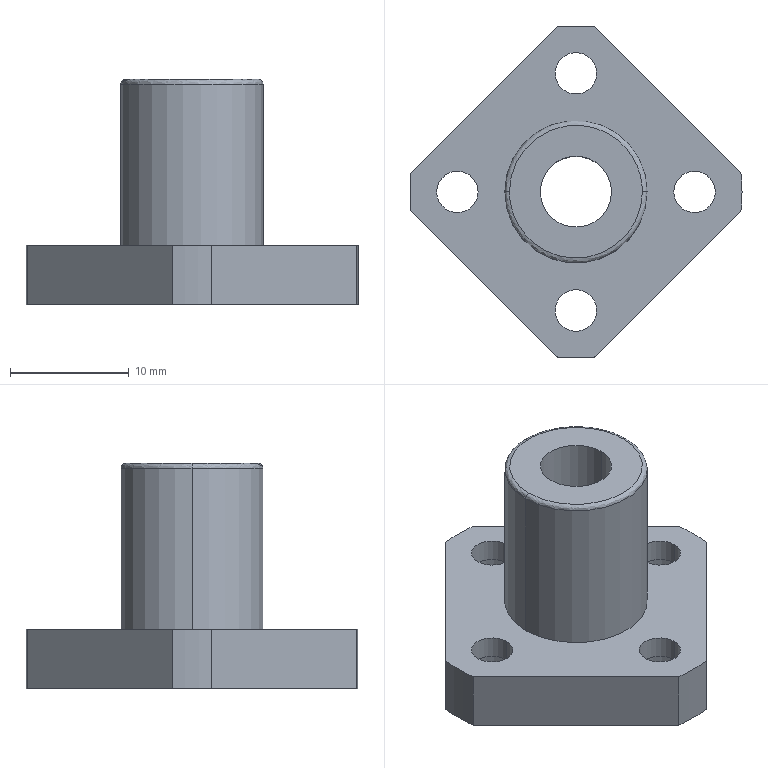Part | SolidWorks | features BaseBody 1 | 1 solid | 38 faces | box 28 x 28 x 19 mm | volume 2991 mm3 | cylinder 25 | plane 11 | spline 2 | commonest cylinder face diameters 6 x10 3.5 x8 28 x5 12 x2
STEP:
#1=CARTESIAN_POINT('',(6.,0.,18.6));
#2=VERTEX_POINT('',#1);
#3=CARTESIAN_POINT('',(-6.,0.,18.6));
#4=VERTEX_POINT('',#3);
#5=CARTESIAN_POINT('',(0.,0.,18.6));
#6=DIRECTION('',(0.,0.,-1.));
#7=DIRECTION('',(1.,0.,0.));
#8=AXIS2_PLACEMENT_3D('',#5,#6,#7);
#9=CIRCLE('',#8,6.);
#10=EDGE_CURVE('',#2,#4,#9,.T.);
#11=ORIENTED_EDGE('',*,*,#10,.F.);
#12=CARTESIAN_POINT('',(5.6,0.,19.));
#13=VERTEX_POINT('',#12);
#14=CARTESIAN_POINT('',(5.6,0.,18.6));
#15=DIRECTION('',(0.,-1.,0.));
#16=DIRECTION('',(1.,0.,0.));
#17=AXIS2_PLACEMENT_3D('',#14,#15,#16);
#18=CIRCLE('',#17,0.4);
#19=EDGE_CURVE('',#2,#13,#18,.T.);
#20=ORIENTED_EDGE('',*,*,#19,.T.);
#21=CARTESIAN_POINT('',(-5.6,0.,19.));
#22=VERTEX_POINT('',#21);
#23=CARTESIAN_POINT('',(5.6,0.,19.));
#24=CARTESIAN_POINT('',(5.6,-11.2,19.));
#25=CARTESIAN_POINT('',(-5.6,-11.2,19.));
#26=CARTESIAN_POINT('',(-5.6,0.,19.));
#27=(BOUNDED_CURVE()B_SPLINE_CURVE(3,(#23,#24,#25,#26),.UNSPECIFIED.,.F.,.T.)B_SPLINE_CURVE_WITH_KNOTS((4,4),(0.5,1.),.UNSPECIFIED.)CURVE()GEOMETRIC_REPRESENTATION_ITEM()RATIONAL_B_SPLINE_CURVE((1.,0.3333,0.3333,1.))REPRESENTATION_ITEM(''));
#28=EDGE_CURVE('',#13,#22,#27,.T.);
#29=ORIENTED_EDGE('',*,*,#28,.T.);
#30=CARTESIAN_POINT('',(-5.6,0.,18.6));
#31=DIRECTION('',(0.,1.,0.));
#32=DIRECTION('',(-1.,0.,0.));
#33=AXIS2_PLACEMENT_3D('',#30,#31,#32);
#34=CIRCLE('',#33,0.4);
#35=EDGE_CURVE('',#4,#22,#34,.T.);
#36=ORIENTED_EDGE('',*,*,#35,.F.);
#37=EDGE_LOOP('',(#11,#20,#29,#36));
#38=FACE_OUTER_BOUND('',#37,.T.);
#39=CARTESIAN_POINT('',(6.,0.,18.6));
#40=CARTESIAN_POINT('',(6.,-12.,18.6));
#41=CARTESIAN_POINT('',(-6.,-12.,18.6));
#42=CARTESIAN_POINT('',(-6.,0.,18.6));
#43=CARTESIAN_POINT('',(6.,0.,18.834));
#44=CARTESIAN_POINT('',(6.,-12.,18.834));
#45=CARTESIAN_POINT('',(-6.,-12.,18.834));
#46=CARTESIAN_POINT('',(-6.,0.,18.834));
#47=CARTESIAN_POINT('',(5.834,0.,19.));
#48=CARTESIAN_POINT('',(5.834,-11.669,19.));
#49=CARTESIAN_POINT('',(-5.834,-11.669,19.));
#50=CARTESIAN_POINT('',(-5.834,0.,19.));
#51=CARTESIAN_POINT('',(5.6,0.,19.));
#52=CARTESIAN_POINT('',(5.6,-11.2,19.));
#53=CARTESIAN_POINT('',(-5.6,-11.2,19.));
#54=CARTESIAN_POINT('',(-5.6,0.,19.));
#55=(BOUNDED_SURFACE()B_SPLINE_SURFACE(3,3,((#39,#40,#41,#42),(#43,#44,#45,#46),(#47,#48,#49,#50),(#51,#52,#53,#54)),.UNSPECIFIED.,.F.,.F.,.F.)B_SPLINE_SURFACE_WITH_KNOTS((4,4),(4,4),(0.,1.),(0.,1.),.UNSPECIFIED.)GEOMETRIC_REPRESENTATION_ITEM()RATIONAL_B_SPLINE_SURFACE(((1.,0.3333,0.3333,1.),(0.8047,0.2682,0.2682,0.8047),(0.8047,0.2682,0.2682,0.8047),(1.,0.3333,0.3333,1.)))REPRESENTATION_ITEM('')SURFACE());
#56=ADVANCED_FACE('',(#38),#55,.T.);
#57=CARTESIAN_POINT('',(6.,0.,5.));
#58=VERTEX_POINT('',#57);
#59=CARTESIAN_POINT('',(-6.,0.,5.));
#60=VERTEX_POINT('',#59);
#61=CARTESIAN_POINT('',(0.,0.,5.));
#62=DIRECTION('',(0.,0.,1.));
#63=DIRECTION('',(1.,0.,0.));
#64=AXIS2_PLACEMENT_3D('',#61,#62,#63);
#65=CIRCLE('',#64,6.);
#66=EDGE_CURVE('',#58,#60,#65,.T.);
#67=ORIENTED_EDGE('',*,*,#66,.T.);
#68=CARTESIAN_POINT('',(-6.,0.,0.));
#69=DIRECTION('',(0.,0.,1.));
#70=VECTOR('',#69,1000.);
#71=LINE('',#68,#70);
#72=EDGE_CURVE('',#60,#4,#71,.T.);
#73=ORIENTED_EDGE('',*,*,#72,.T.);
#74=CARTESIAN_POINT('',(0.,0.,18.6));
#75=DIRECTION('',(0.,0.,-1.));
#76=DIRECTION('',(1.,0.,0.));
#77=AXIS2_PLACEMENT_3D('',#74,#75,#76);
#78=CIRCLE('',#77,6.);
#79=EDGE_CURVE('',#4,#2,#78,.T.);
#80=ORIENTED_EDGE('',*,*,#79,.T.);
#81=CARTESIAN_POINT('',(6.,0.,0.));
#82=DIRECTION('',(0.,0.,1.));
#83=VECTOR('',#82,1000.);
#84=LINE('',#81,#83);
#85=EDGE_CURVE('',#58,#2,#84,.T.);
#86=ORIENTED_EDGE('',*,*,#85,.F.);
#87=EDGE_LOOP('',(#67,#73,#80,#86));
#88=FACE_OUTER_BOUND('',#87,.T.);
#89=CARTESIAN_POINT('',(0.,0.,0.));
#90=DIRECTION('',(0.,0.,1.));
#91=DIRECTION('',(1.,0.,0.));
#92=AXIS2_PLACEMENT_3D('',#89,#90,#91);
#93=CYLINDRICAL_SURFACE('',#92,6.);
#94=ADVANCED_FACE('',(#88),#93,.T.);
#95=CARTESIAN_POINT('',(-1.75,10.,3.1));
#96=VERTEX_POINT('',#95);
#97=CARTESIAN_POINT('',(1.75,10.,3.1));
#98=VERTEX_POINT('',#97);
#99=CARTESIAN_POINT('',(0.,10.,3.1));
#100=DIRECTION('',(0.,0.,1.));
#101=DIRECTION('',(1.,0.,0.));
#102=AXIS2_PLACEMENT_3D('',#99,#100,#101);
#103=CIRCLE('',#102,1.75);
#104=EDGE_CURVE('',#96,#98,#103,.T.);
#105=ORIENTED_EDGE('',*,*,#104,.F.);
#106=CARTESIAN_POINT('',(-1.75,10.,5.));
#107=VERTEX_POINT('',#106);
#108=CARTESIAN_POINT('',(-1.75,10.,0.));
#109=DIRECTION('',(0.,0.,1.));
#110=VECTOR('',#109,1000.);
#111=LINE('',#108,#110);
#112=EDGE_CURVE('',#96,#107,#111,.T.);
#113=ORIENTED_EDGE('',*,*,#112,.T.);
#114=CARTESIAN_POINT('',(1.75,10.,5.));
#115=VERTEX_POINT('',#114);
#116=CARTESIAN_POINT('',(0.,10.,5.));
#117=DIRECTION('',(0.,0.,-1.));
#118=DIRECTION('',(1.,0.,0.));
#119=AXIS2_PLACEMENT_3D('',#116,#117,#118);
#120=CIRCLE('',#119,1.75);
#121=EDGE_CURVE('',#115,#107,#120,.T.);
#122=ORIENTED_EDGE('',*,*,#121,.F.);
#123=CARTESIAN_POINT('',(1.75,10.,0.));
#124=DIRECTION('',(0.,0.,1.));
#125=VECTOR('',#124,1000.);
#126=LINE('',#123,#125);
#127=EDGE_CURVE('',#98,#115,#126,.T.);
#128=ORIENTED_EDGE('',*,*,#127,.F.);
#129=EDGE_LOOP('',(#105,#113,#122,#128));
#130=FACE_OUTER_BOUND('',#129,.T.);
#131=CARTESIAN_POINT('',(0.,10.,0.));
#132=DIRECTION('',(0.,0.,1.));
#133=DIRECTION('',(1.,0.,0.));
#134=AXIS2_PLACEMENT_3D('',#131,#132,#133);
#135=CYLINDRICAL_SURFACE('',#134,1.75);
#136=ADVANCED_FACE('',(#130),#135,.F.);
#137=CARTESIAN_POINT('',(11.75,0.,5.));
#138=VERTEX_POINT('',#137);
#139=CARTESIAN_POINT('',(8.25,0.,5.));
#140=VERTEX_POINT('',#139);
#141=CARTESIAN_POINT('',(10.,0.,5.));
#142=DIRECTION('',(0.,0.,-1.));
#143=DIRECTION('',(-1.,0.,0.));
#144=AXIS2_PLACEMENT_3D('',#141,#142,#143);
#145=CIRCLE('',#144,1.75);
#146=EDGE_CURVE('',#138,#140,#145,.T.);
#147=ORIENTED_EDGE('',*,*,#146,.F.);
#148=CARTESIAN_POINT('',(11.75,0.,3.1));
#149=VERTEX_POINT('',#148);
#150=CARTESIAN_POINT('',(11.75,0.,5.));
#151=DIRECTION('',(0.,0.,-1.));
#152=VECTOR('',#151,1000.);
#153=LINE('',#150,#152);
#154=EDGE_CURVE('',#138,#149,#153,.T.);
#155=ORIENTED_EDGE('',*,*,#154,.T.);
#156=CARTESIAN_POINT('',(8.25,0.,3.1));
#157=VERTEX_POINT('',#156);
#158=CARTESIAN_POINT('',(10.,0.,3.1));
#159=DIRECTION('',(0.,0.,1.));
#160=DIRECTION('',(-1.,0.,0.));
#161=AXIS2_PLACEMENT_3D('',#158,#159,#160);
#162=CIRCLE('',#161,1.75);
#163=EDGE_CURVE('',#157,#149,#162,.T.);
#164=ORIENTED_EDGE('',*,*,#163,.F.);
#165=CARTESIAN_POINT('',(8.25,0.,5.));
#166=DIRECTION('',(0.,0.,-1.));
#167=VECTOR('',#166,1000.);
#168=LINE('',#165,#167);
#169=EDGE_CURVE('',#140,#157,#168,.T.);
#170=ORIENTED_EDGE('',*,*,#169,.F.);
#171=EDGE_LOOP('',(#147,#155,#164,#170));
#172=FACE_OUTER_BOUND('',#171,.T.);
#173=CARTESIAN_POINT('',(10.,0.,5.));
#174=DIRECTION('',(0.,0.,-1.));
#175=DIRECTION('',(-1.,0.,0.));
#176=AXIS2_PLACEMENT_3D('',#173,#174,#175);
#177=CYLINDRICAL_SURFACE('',#176,1.75);
#178=ADVANCED_FACE('',(#172),#177,.F.);
#179=CARTESIAN_POINT('',(13.902,-1.654,0.));
#180=VERTEX_POINT('',#179);
#181=CARTESIAN_POINT('',(14.,0.,0.));
#182=VERTEX_POINT('',#181);
#183=CARTESIAN_POINT('',(0.,0.,0.));
#184=DIRECTION('',(0.,0.,1.));
#185=DIRECTION('',(1.,0.,0.));
#186=AXIS2_PLACEMENT_3D('',#183,#184,#185);
#187=CIRCLE('',#186,14.);
#188=EDGE_CURVE('',#180,#182,#187,.T.);
#189=ORIENTED_EDGE('',*,*,#188,.T.);
#190=CARTESIAN_POINT('',(14.,0.,5.));
#191=VERTEX_POINT('',#190);
#192=CARTESIAN_POINT('',(14.,0.,5.));
#193=DIRECTION('',(0.,0.,1.));
#194=VECTOR('',#193,1000.);
#195=LINE('',#192,#194);
#196=EDGE_CURVE('',#182,#191,#195,.T.);
#197=ORIENTED_EDGE('',*,*,#196,.T.);
#198=CARTESIAN_POINT('',(13.902,-1.654,5.));
#199=VERTEX_POINT('',#198);
#200=CARTESIAN_POINT('',(0.,0.,5.));
#201=DIRECTION('',(0.,0.,1.));
#202=DIRECTION('',(1.,0.,0.));
#203=AXIS2_PLACEMENT_3D('',#200,#201,#202);
#204=CIRCLE('',#203,14.);
#205=EDGE_CURVE('',#199,#191,#204,.T.);
#206=ORIENTED_EDGE('',*,*,#205,.F.);
#207=CARTESIAN_POINT('',(13.902,-1.654,5.));
#208=DIRECTION('',(0.,0.,-1.));
#209=VECTOR('',#208,1000.);
#210=LINE('',#207,#209);
#211=EDGE_CURVE('',#199,#180,#210,.T.);
#212=ORIENTED_EDGE('',*,*,#211,.T.);
#213=EDGE_LOOP('',(#189,#197,#206,#212));
#214=FACE_OUTER_BOUND('',#213,.T.);
#215=CARTESIAN_POINT('',(0.,0.,5.));
#216=DIRECTION('',(0.,0.,1.));
#217=DIRECTION('',(1.,0.,0.));
#218=AXIS2_PLACEMENT_3D('',#215,#216,#217);
#219=CYLINDRICAL_SURFACE('',#218,14.);
#220=ADVANCED_FACE('',(#214),#219,.T.);
#221=CARTESIAN_POINT('',(-11.75,0.,3.1));
#222=VERTEX_POINT('',#221);
#223=CARTESIAN_POINT('',(-8.25,0.,3.1));
#224=VERTEX_POINT('',#223);
#225=CARTESIAN_POINT('',(-10.,0.,3.1));
#226=DIRECTION('',(0.,0.,1.));
#227=DIRECTION('',(1.,0.,0.));
#228=AXIS2_PLACEMENT_3D('',#225,#226,#227);
#229=CIRCLE('',#228,1.75);
#230=EDGE_CURVE('',#222,#224,#229,.T.);
#231=ORIENTED_EDGE('',*,*,#230,.F.);
#232=CARTESIAN_POINT('',(-11.75,0.,5.));
#233=VERTEX_POINT('',#232);
#234=CARTESIAN_POINT('',(-11.75,0.,0.));
#235=DIRECTION('',(0.,0.,1.));
#236=VECTOR('',#235,1000.);
#237=LINE('',#234,#236);
#238=EDGE_CURVE('',#222,#233,#237,.T.);
#239=ORIENTED_EDGE('',*,*,#238,.T.);
#240=CARTESIAN_POINT('',(-8.25,0.,5.));
#241=VERTEX_POINT('',#240);
#242=CARTESIAN_POINT('',(-10.,0.,5.));
#243=DIRECTION('',(0.,0.,-1.));
#244=DIRECTION('',(1.,0.,0.));
#245=AXIS2_PLACEMENT_3D('',#242,#243,#244);
#246=CIRCLE('',#245,1.75);
#247=EDGE_CURVE('',#241,#233,#246,.T.);
#248=ORIENTED_EDGE('',*,*,#247,.F.);
#249=CARTESIAN_POINT('',(-8.25,0.,0.));
#250=DIRECTION('',(0.,0.,1.));
#251=VECTOR('',#250,1000.);
#252=LINE('',#249,#251);
#253=EDGE_CURVE('',#224,#241,#252,.T.);
#254=ORIENTED_EDGE('',*,*,#253,.F.);
#255=EDGE_LOOP('',(#231,#239,#248,#254));
#256=FACE_OUTER_BOUND('',#255,.T.);
#257=CARTESIAN_POINT('',(-10.,0.,0.));
#258=DIRECTION('',(0.,0.,1.));
#259=DIRECTION('',(1.,0.,0.));
#260=AXIS2_PLACEMENT_3D('',#257,#258,#259);
#261=CYLINDRICAL_SURFACE('',#260,1.75);
#262=ADVANCED_FACE('',(#256),#261,.F.);
#263=CARTESIAN_POINT('',(1.75,-10.,5.));
#264=VERTEX_POINT('',#263);
#265=CARTESIAN_POINT('',(-1.75,-10.,5.));
#266=VERTEX_POINT('',#265);
#267=CARTESIAN_POINT('',(0.,-10.,5.));
#268=DIRECTION('',(0.,0.,-1.));
#269=DIRECTION('',(-1.,0.,0.));
#270=AXIS2_PLACEMENT_3D('',#267,#268,#269);
#271=CIRCLE('',#270,1.75);
#272=EDGE_CURVE('',#264,#266,#271,.T.);
#273=ORIENTED_EDGE('',*,*,#272,.F.);
#274=CARTESIAN_POINT('',(1.75,-10.,3.1));
#275=VERTEX_POINT('',#274);
#276=CARTESIAN_POINT('',(1.75,-10.,5.));
#277=DIRECTION('',(0.,0.,-1.));
#278=VECTOR('',#277,1000.);
#279=LINE('',#276,#278);
#280=EDGE_CURVE('',#264,#275,#279,.T.);
#281=ORIENTED_EDGE('',*,*,#280,.T.);
#282=CARTESIAN_POINT('',(-1.75,-10.,3.1));
#283=VERTEX_POINT('',#282);
#284=CARTESIAN_POINT('',(0.,-10.,3.1));
#285=DIRECTION('',(0.,0.,1.));
#286=DIRECTION('',(-1.,0.,0.));
#287=AXIS2_PLACEMENT_3D('',#284,#285,#286);
#288=CIRCLE('',#287,1.75);
#289=EDGE_CURVE('',#283,#275,#288,.T.);
#290=ORIENTED_EDGE('',*,*,#289,.F.);
#291=CARTESIAN_POINT('',(-1.75,-10.,5.));
#292=DIRECTION('',(0.,0.,-1.));
#293=VECTOR('',#292,1000.);
#294=LINE('',#291,#293);
#295=EDGE_CURVE('',#266,#283,#294,.T.);
#296=ORIENTED_EDGE('',*,*,#295,.F.);
#297=EDGE_LOOP('',(#273,#281,#290,#296));
#298=FACE_OUTER_BOUND('',#297,.T.);
#299=CARTESIAN_POINT('',(0.,-10.,5.));
#300=DIRECTION('',(0.,0.,-1.));
#301=DIRECTION('',(-1.,0.,0.));
#302=AXIS2_PLACEMENT_3D('',#299,#300,#301);
#303=CYLINDRICAL_SURFACE('',#302,1.75);
#304=ADVANCED_FACE('',(#298),#303,.F.);
#305=CARTESIAN_POINT('',(-3.,0.,0.));
#306=VERTEX_POINT('',#305);
#307=CARTESIAN_POINT('',(3.,0.,0.));
#308=VERTEX_POINT('',#307);
#309=CARTESIAN_POINT('',(0.,0.,0.));
#310=DIRECTION('',(0.,0.,1.));
#311=DIRECTION('',(1.,0.,0.));
#312=AXIS2_PLACEMENT_3D('',#309,#310,#311);
#313=CIRCLE('',#312,3.);
#314=EDGE_CURVE('',#306,#308,#313,.T.);
#315=ORIENTED_EDGE('',*,*,#314,.F.);
#316=CARTESIAN_POINT('',(-3.,0.,19.));
#317=VERTEX_POINT('',#316);
#318=CARTESIAN_POINT('',(-3.,0.,0.));
#319=DIRECTION('',(0.,0.,1.));
#320=VECTOR('',#319,1000.);
#321=LINE('',#318,#320);
#322=EDGE_CURVE('',#306,#317,#321,.T.);
#323=ORIENTED_EDGE('',*,*,#322,.T.);
#324=CARTESIAN_POINT('',(3.,0.,19.));
#325=VERTEX_POINT('',#324);
#326=CARTESIAN_POINT('',(0.,0.,19.));
#327=DIRECTION('',(0.,0.,-1.));
#328=DIRECTION('',(1.,0.,0.));
#329=AXIS2_PLACEMENT_3D('',#326,#327,#328);
#330=CIRCLE('',#329,3.);
#331=EDGE_CURVE('',#325,#317,#330,.T.);
#332=ORIENTED_EDGE('',*,*,#331,.F.);
#333=CARTESIAN_POINT('',(3.,0.,0.));
#334=DIRECTION('',(0.,0.,1.));
#335=VECTOR('',#334,1000.);
#336=LINE('',#333,#335);
#337=EDGE_CURVE('',#308,#325,#336,.T.);
#338=ORIENTED_EDGE('',*,*,#337,.F.);
#339=EDGE_LOOP('',(#315,#323,#332,#338));
#340=FACE_OUTER_BOUND('',#339,.T.);
#341=CARTESIAN_POINT('',(0.,0.,0.));
#342=DIRECTION('',(0.,0.,1.));
#343=DIRECTION('',(1.,0.,0.));
#344=AXIS2_PLACEMENT_3D('',#341,#342,#343);
#345=CYLINDRICAL_SURFACE('',#344,3.);
#346=ADVANCED_FACE('',(#340),#345,.F.);
#347=CARTESIAN_POINT('',(-3.,10.,0.));
#348=VERTEX_POINT('',#347);
#349=CARTESIAN_POINT('',(3.,10.,0.));
#350=VERTEX_POINT('',#349);
#351=CARTESIAN_POINT('',(0.,10.,0.));
#352=DIRECTION('',(0.,0.,1.));
#353=DIRECTION('',(1.,0.,0.));
#354=AXIS2_PLACEMENT_3D('',#351,#352,#353);
#355=CIRCLE('',#354,3.);
#356=EDGE_CURVE('',#348,#350,#355,.T.);
#357=ORIENTED_EDGE('',*,*,#356,.F.);
#358=CARTESIAN_POINT('',(-3.,10.,3.1));
#359=VERTEX_POINT('',#358);
#360=CARTESIAN_POINT('',(-3.,10.,0.));
#361=DIRECTION('',(0.,0.,1.));
#362=VECTOR('',#361,1000.);
#363=LINE('',#360,#362);
#364=EDGE_CURVE('',#348,#359,#363,.T.);
#365=ORIENTED_EDGE('',*,*,#364,.T.);
#366=CARTESIAN_POINT('',(3.,10.,3.1));
#367=VERTEX_POINT('',#366);
#368=CARTESIAN_POINT('',(0.,10.,3.1));
#369=DIRECTION('',(0.,0.,-1.));
#370=DIRECTION('',(1.,0.,0.));
#371=AXIS2_PLACEMENT_3D('',#368,#369,#370);
#372=CIRCLE('',#371,3.);
#373=EDGE_CURVE('',#367,#359,#372,.T.);
#374=ORIENTED_EDGE('',*,*,#373,.F.);
#375=CARTESIAN_POINT('',(3.,10.,0.));
#376=DIRECTION('',(0.,0.,1.));
#377=VECTOR('',#376,1000.);
#378=LINE('',#375,#377);
#379=EDGE_CURVE('',#350,#367,#378,.T.);
#380=ORIENTED_EDGE('',*,*,#379,.F.);
#381=EDGE_LOOP('',(#357,#365,#374,#380));
#382=FACE_OUTER_BOUND('',#381,.T.);
#383=CARTESIAN_POINT('',(0.,10.,0.));
#384=DIRECTION('',(0.,0.,1.));
#385=DIRECTION('',(1.,0.,0.));
#386=AXIS2_PLACEMENT_3D('',#383,#384,#385);
#387=CYLINDRICAL_SURFACE('',#386,3.);
#388=ADVANCED_FACE('',(#382),#387,.F.);
#389=CARTESIAN_POINT('',(13.,0.,3.1));
#390=VERTEX_POINT('',#389);
#391=CARTESIAN_POINT('',(7.,0.,3.1));
#392=VERTEX_POINT('',#391);
#393=CARTESIAN_POINT('',(10.,0.,3.1));
#394=DIRECTION('',(0.,0.,-1.));
#395=DIRECTION('',(-1.,0.,0.));
#396=AXIS2_PLACEMENT_3D('',#393,#394,#395);
#397=CIRCLE('',#396,3.);
#398=EDGE_CURVE('',#390,#392,#397,.T.);
#399=ORIENTED_EDGE('',*,*,#398,.F.);
#400=CARTESIAN_POINT('',(13.,0.,0.));
#401=VERTEX_POINT('',#400);
#402=CARTESIAN_POINT('',(13.,0.,5.));
#403=DIRECTION('',(0.,0.,-1.));
#404=VECTOR('',#403,1000.);
#405=LINE('',#402,#404);
#406=EDGE_CURVE('',#390,#401,#405,.T.);
#407=ORIENTED_EDGE('',*,*,#406,.T.);
#408=CARTESIAN_POINT('',(7.,0.,0.));
#409=VERTEX_POINT('',#408);
#410=CARTESIAN_POINT('',(10.,0.,0.));
#411=DIRECTION('',(0.,0.,1.));
#412=DIRECTION('',(-1.,0.,0.));
#413=AXIS2_PLACEMENT_3D('',#410,#411,#412);
#414=CIRCLE('',#413,3.);
#415=EDGE_CURVE('',#409,#401,#414,.T.);
#416=ORIENTED_EDGE('',*,*,#415,.F.);
#417=CARTESIAN_POINT('',(7.,0.,5.));
#418=DIRECTION('',(0.,0.,-1.));
#419=VECTOR('',#418,1000.);
#420=LINE('',#417,#419);
#421=EDGE_CURVE('',#392,#409,#420,.T.);
#422=ORIENTED_EDGE('',*,*,#421,.F.);
#423=EDGE_LOOP('',(#399,#407,#416,#422));
#424=FACE_OUTER_BOUND('',#423,.T.);
#425=CARTESIAN_POINT('',(10.,0.,5.));
#426=DIRECTION('',(0.,0.,-1.));
#427=DIRECTION('',(-1.,0.,0.));
#428=AXIS2_PLACEMENT_3D('',#425,#426,#427);
#429=CYLINDRICAL_SURFACE('',#428,3.);
#430=ADVANCED_FACE('',(#424),#429,.F.);
#431=CARTESIAN_POINT('',(-13.,0.,0.));
#432=VERTEX_POINT('',#431);
#433=CARTESIAN_POINT('',(-7.,0.,0.));
#434=VERTEX_POINT('',#433);
#435=CARTESIAN_POINT('',(-10.,0.,0.));
#436=DIRECTION('',(0.,0.,1.));
#437=DIRECTION('',(1.,0.,0.));
#438=AXIS2_PLACEMENT_3D('',#435,#436,#437);
#439=CIRCLE('',#438,3.);
#440=EDGE_CURVE('',#432,#434,#439,.T.);
#441=ORIENTED_EDGE('',*,*,#440,.F.);
#442=CARTESIAN_POINT('',(-13.,0.,3.1));
#443=VERTEX_POINT('',#442);
#444=CARTESIAN_POINT('',(-13.,0.,0.));
#445=DIRECTION('',(0.,0.,1.));
#446=VECTOR('',#445,1000.);
#447=LINE('',#444,#446);
#448=EDGE_CURVE('',#432,#443,#447,.T.);
#449=ORIENTED_EDGE('',*,*,#448,.T.);
#450=CARTESIAN_POINT('',(-7.,0.,3.1));
#451=VERTEX_POINT('',#450);
#452=CARTESIAN_POINT('',(-10.,0.,3.1));
#453=DIRECTION('',(0.,0.,-1.));
#454=DIRECTION('',(1.,0.,0.));
#455=AXIS2_PLACEMENT_3D('',#452,#453,#454);
#456=CIRCLE('',#455,3.);
#457=EDGE_CURVE('',#451,#443,#456,.T.);
#458=ORIENTED_EDGE('',*,*,#457,.F.);
#459=CARTESIAN_POINT('',(-7.,0.,0.));
#460=DIRECTION('',(0.,0.,1.));
#461=VECTOR('',#460,1000.);
#462=LINE('',#459,#461);
#463=EDGE_CURVE('',#434,#451,#462,.T.);
#464=ORIENTED_EDGE('',*,*,#463,.F.);
#465=EDGE_LOOP('',(#441,#449,#458,#464));
#466=FACE_OUTER_BOUND('',#465,.T.);
#467=CARTESIAN_POINT('',(-10.,0.,0.));
#468=DIRECTION('',(0.,0.,1.));
#469=DIRECTION('',(1.,0.,0.));
#470=AXIS2_PLACEMENT_3D('',#467,#468,#469);
#471=CYLINDRICAL_SURFACE('',#470,3.);
#472=ADVANCED_FACE('',(#466),#471,.F.);
#473=CARTESIAN_POINT('',(3.,-10.,3.1));
#474=VERTEX_POINT('',#473);
#475=CARTESIAN_POINT('',(-3.,-10.,3.1));
#476=VERTEX_POINT('',#475);
#477=CARTESIAN_POINT('',(0.,-10.,3.1));
#478=DIRECTION('',(0.,0.,-1.));
#479=DIRECTION('',(-1.,0.,0.));
#480=AXIS2_PLACEMENT_3D('',#477,#478,#479);
#481=CIRCLE('',#480,3.);
#482=EDGE_CURVE('',#474,#476,#481,.T.);
#483=ORIENTED_EDGE('',*,*,#482,.F.);
#484=CARTESIAN_POINT('',(3.,-10.,0.));
#485=VERTEX_POINT('',#484);
#486=CARTESIAN_POINT('',(3.,-10.,5.));
#487=DIRECTION('',(0.,0.,-1.));
#488=VECTOR('',#487,1000.);
#489=LINE('',#486,#488);
#490=EDGE_CURVE('',#474,#485,#489,.T.);
#491=ORIENTED_EDGE('',*,*,#490,.T.);
#492=CARTESIAN_POINT('',(-3.,-10.,0.));
#493=VERTEX_POINT('',#492);
#494=CARTESIAN_POINT('',(0.,-10.,0.));
#495=DIRECTION('',(0.,0.,1.));
#496=DIRECTION('',(-1.,0.,0.));
#497=AXIS2_PLACEMENT_3D('',#494,#495,#496);
#498=CIRCLE('',#497,3.);
#499=EDGE_CURVE('',#493,#485,#498,.T.);
#500=ORIENTED_EDGE('',*,*,#499,.F.);
#501=CARTESIAN_POINT('',(-3.,-10.,5.));
#502=DIRECTION('',(0.,0.,-1.));
#503=VECTOR('',#502,1000.);
#504=LINE('',#501,#503);
#505=EDGE_CURVE('',#476,#493,#504,.T.);
#506=ORIENTED_EDGE('',*,*,#505,.F.);
#507=EDGE_LOOP('',(#483,#491,#500,#506));
#508=FACE_OUTER_BOUND('',#507,.T.);
#509=CARTESIAN_POINT('',(0.,-10.,5.));
#510=DIRECTION('',(0.,0.,-1.));
#511=DIRECTION('',(-1.,0.,0.));
#512=AXIS2_PLACEMENT_3D('',#509,#510,#511);
#513=CYLINDRICAL_SURFACE('',#512,3.);
#514=ADVANCED_FACE('',(#508),#513,.F.);
#515=ORIENTED_EDGE('',*,*,#72,.F.);
#516=CARTESIAN_POINT('',(0.,0.,5.));
#517=DIRECTION('',(0.,0.,1.));
#518=DIRECTION('',(1.,0.,0.));
#519=AXIS2_PLACEMENT_3D('',#516,#517,#518);
#520=CIRCLE('',#519,6.);
#521=EDGE_CURVE('',#60,#58,#520,.T.);
#522=ORIENTED_EDGE('',*,*,#521,.T.);
#523=ORIENTED_EDGE('',*,*,#85,.T.);
#524=ORIENTED_EDGE('',*,*,#10,.T.);
#525=EDGE_LOOP('',(#515,#522,#523,#524));
#526=FACE_OUTER_BOUND('',#525,.T.);
#527=CARTESIAN_POINT('',(0.,0.,0.));
#528=DIRECTION('',(0.,0.,1.));
#529=DIRECTION('',(1.,0.,0.));
#530=AXIS2_PLACEMENT_3D('',#527,#528,#529);
#531=CYLINDRICAL_SURFACE('',#530,6.);
#532=ADVANCED_FACE('',(#526),#531,.T.);
#533=ORIENTED_EDGE('',*,*,#121,.T.);
#534=CARTESIAN_POINT('',(0.,10.,5.));
#535=DIRECTION('',(0.,0.,-1.));
#536=DIRECTION('',(1.,0.,0.));
#537=AXIS2_PLACEMENT_3D('',#534,#535,#536);
#538=CIRCLE('',#537,1.75);
#539=EDGE_CURVE('',#107,#115,#538,.T.);
#540=ORIENTED_EDGE('',*,*,#539,.T.);
#541=EDGE_LOOP('',(#533,#540));
#542=FACE_BOUND('',#541,.T.);
#543=CARTESIAN_POINT('',(10.,0.,5.));
#544=DIRECTION('',(0.,0.,-1.));
#545=DIRECTION('',(-1.,0.,0.));
#546=AXIS2_PLACEMENT_3D('',#543,#544,#545);
#547=CIRCLE('',#546,1.75);
#548=EDGE_CURVE('',#140,#138,#547,.T.);
#549=ORIENTED_EDGE('',*,*,#548,.T.);
#550=ORIENTED_EDGE('',*,*,#146,.T.);
#551=EDGE_LOOP('',(#549,#550));
#552=FACE_BOUND('',#551,.T.);
#553=CARTESIAN_POINT('',(13.902,1.654,5.));
#554=VERTEX_POINT('',#553);
#555=CARTESIAN_POINT('',(1.654,13.902,5.));
#556=VERTEX_POINT('',#555);
#557=CARTESIAN_POINT('',(13.902,1.654,5.));
#558=DIRECTION('',(-0.7071,0.7071,0.));
#559=VECTOR('',#558,1000.);
#560=LINE('',#557,#559);
#561=EDGE_CURVE('',#554,#556,#560,.T.);
#562=ORIENTED_EDGE('',*,*,#561,.T.);
#563=CARTESIAN_POINT('',(-1.654,13.902,5.));
#564=VERTEX_POINT('',#563);
#565=CARTESIAN_POINT('',(0.,0.,5.));
#566=DIRECTION('',(0.,0.,1.));
#567=DIRECTION('',(1.,0.,0.));
#568=AXIS2_PLACEMENT_3D('',#565,#566,#567);
#569=CIRCLE('',#568,14.);
#570=EDGE_CURVE('',#556,#564,#569,.T.);
#571=ORIENTED_EDGE('',*,*,#570,.T.);
#572=CARTESIAN_POINT('',(-13.902,1.654,5.));
#573=VERTEX_POINT('',#572);
#574=CARTESIAN_POINT('',(-1.654,13.902,5.));
#575=DIRECTION('',(-0.7071,-0.7071,0.));
#576=VECTOR('',#575,1000.);
#577=LINE('',#574,#576);
#578=EDGE_CURVE('',#564,#573,#577,.T.);
#579=ORIENTED_EDGE('',*,*,#578,.T.);
#580=CARTESIAN_POINT('',(-13.902,-1.654,5.));
#581=VERTEX_POINT('',#580);
#582=CARTESIAN_POINT('',(0.,0.,5.));
#583=DIRECTION('',(0.,0.,1.));
#584=DIRECTION('',(1.,0.,0.));
#585=AXIS2_PLACEMENT_3D('',#582,#583,#584);
#586=CIRCLE('',#585,14.);
#587=EDGE_CURVE('',#573,#581,#586,.T.);
#588=ORIENTED_EDGE('',*,*,#587,.T.);
#589=CARTESIAN_POINT('',(-1.654,-13.902,5.));
#590=VERTEX_POINT('',#589);
#591=CARTESIAN_POINT('',(-13.902,-1.654,5.));
#592=DIRECTION('',(0.7071,-0.7071,0.));
#593=VECTOR('',#592,1000.);
#594=LINE('',#591,#593);
#595=EDGE_CURVE('',#581,#590,#594,.T.);
#596=ORIENTED_EDGE('',*,*,#595,.T.);
#597=CARTESIAN_POINT('',(1.654,-13.902,5.));
#598=VERTEX_POINT('',#597);
#599=CARTESIAN_POINT('',(0.,0.,5.));
#600=DIRECTION('',(0.,0.,1.));
#601=DIRECTION('',(1.,0.,0.));
#602=AXIS2_PLACEMENT_3D('',#599,#600,#601);
#603=CIRCLE('',#602,14.);
#604=EDGE_CURVE('',#590,#598,#603,.T.);
#605=ORIENTED_EDGE('',*,*,#604,.T.);
#606=CARTESIAN_POINT('',(1.654,-13.902,5.));
#607=DIRECTION('',(0.7071,0.7071,0.));
#608=VECTOR('',#607,1000.);
#609=LINE('',#606,#608);
#610=EDGE_CURVE('',#598,#199,#609,.T.);
#611=ORIENTED_EDGE('',*,*,#610,.T.);
#612=ORIENTED_EDGE('',*,*,#205,.T.);
#613=CARTESIAN_POINT('',(0.,0.,5.));
#614=DIRECTION('',(0.,0.,1.));
#615=DIRECTION('',(1.,0.,0.));
#616=AXIS2_PLACEMENT_3D('',#613,#614,#615);
#617=CIRCLE('',#616,14.);
#618=EDGE_CURVE('',#191,#554,#617,.T.);
#619=ORIENTED_EDGE('',*,*,#618,.T.);
#620=EDGE_LOOP('',(#562,#571,#579,#588,#596,#605,#611,#612,#619));
#621=FACE_OUTER_BOUND('',#620,.T.);
#622=ORIENTED_EDGE('',*,*,#66,.F.);
#623=ORIENTED_EDGE('',*,*,#521,.F.);
#624=EDGE_LOOP('',(#622,#623));
#625=FACE_BOUND('',#624,.T.);
#626=ORIENTED_EDGE('',*,*,#247,.T.);
#627=CARTESIAN_POINT('',(-10.,0.,5.));
#628=DIRECTION('',(0.,0.,-1.));
#629=DIRECTION('',(1.,0.,0.));
#630=AXIS2_PLACEMENT_3D('',#627,#628,#629);
#631=CIRCLE('',#630,1.75);
#632=EDGE_CURVE('',#233,#241,#631,.T.);
#633=ORIENTED_EDGE('',*,*,#632,.T.);
#634=EDGE_LOOP('',(#626,#633));
#635=FACE_BOUND('',#634,.T.);
#636=CARTESIAN_POINT('',(0.,-10.,5.));
#637=DIRECTION('',(0.,0.,-1.));
#638=DIRECTION('',(-1.,0.,0.));
#639=AXIS2_PLACEMENT_3D('',#636,#637,#638);
#640=CIRCLE('',#639,1.75);
#641=EDGE_CURVE('',#266,#264,#640,.T.);
#642=ORIENTED_EDGE('',*,*,#641,.T.);
#643=ORIENTED_EDGE('',*,*,#272,.T.);
#644=EDGE_LOOP('',(#642,#643));
#645=FACE_BOUND('',#644,.T.);
#646=CARTESIAN_POINT('',(0.,0.,5.));
#647=DIRECTION('',(0.,0.,1.));
#648=DIRECTION('',(1.,0.,0.));
#649=AXIS2_PLACEMENT_3D('',#646,#647,#648);
#650=PLANE('',#649);
#651=ADVANCED_FACE('',(#542,#552,#621,#625,#635,#645),#650,.T.);
#652=ORIENTED_EDGE('',*,*,#19,.F.);
#653=ORIENTED_EDGE('',*,*,#79,.F.);
#654=ORIENTED_EDGE('',*,*,#35,.T.);
#655=CARTESIAN_POINT('',(-5.6,0.,19.));
#656=CARTESIAN_POINT('',(-5.6,11.2,19.));
#657=CARTESIAN_POINT('',(5.6,11.2,19.));
#658=CARTESIAN_POINT('',(5.6,0.,19.));
#659=(BOUNDED_CURVE()B_SPLINE_CURVE(3,(#655,#656,#657,#658),.UNSPECIFIED.,.F.,.T.)B_SPLINE_CURVE_WITH_KNOTS((4,4),(0.,0.5),.UNSPECIFIED.)CURVE()GEOMETRIC_REPRESENTATION_ITEM()RATIONAL_B_SPLINE_CURVE((1.,0.3333,0.3333,1.))REPRESENTATION_ITEM(''));
#660=EDGE_CURVE('',#22,#13,#659,.T.);
#661=ORIENTED_EDGE('',*,*,#660,.T.);
#662=EDGE_LOOP('',(#652,#653,#654,#661));
#663=FACE_OUTER_BOUND('',#662,.T.);
#664=CARTESIAN_POINT('',(-6.,0.,18.6));
#665=CARTESIAN_POINT('',(-6.,12.,18.6));
#666=CARTESIAN_POINT('',(6.,12.,18.6));
#667=CARTESIAN_POINT('',(6.,0.,18.6));
#668=CARTESIAN_POINT('',(-6.,0.,18.834));
#669=CARTESIAN_POINT('',(-6.,12.,18.834));
#670=CARTESIAN_POINT('',(6.,12.,18.834));
#671=CARTESIAN_POINT('',(6.,0.,18.834));
#672=CARTESIAN_POINT('',(-5.834,0.,19.));
#673=CARTESIAN_POINT('',(-5.834,11.669,19.));
#674=CARTESIAN_POINT('',(5.834,11.669,19.));
#675=CARTESIAN_POINT('',(5.834,0.,19.));
#676=CARTESIAN_POINT('',(-5.6,0.,19.));
#677=CARTESIAN_POINT('',(-5.6,11.2,19.));
#678=CARTESIAN_POINT('',(5.6,11.2,19.));
#679=CARTESIAN_POINT('',(5.6,0.,19.));
#680=(BOUNDED_SURFACE()B_SPLINE_SURFACE(3,3,((#664,#665,#666,#667),(#668,#669,#670,#671),(#672,#673,#674,#675),(#676,#677,#678,#679)),.UNSPECIFIED.,.F.,.F.,.T.)B_SPLINE_SURFACE_WITH_KNOTS((4,4),(4,4),(0.,1.),(0.,1.),.UNSPECIFIED.)GEOMETRIC_REPRESENTATION_ITEM()RATIONAL_B_SPLINE_SURFACE(((1.,0.3333,0.3333,1.),(0.8047,0.2682,0.2682,0.8047),(0.8047,0.2682,0.2682,0.8047),(1.,0.3333,0.3333,1.)))REPRESENTATION_ITEM('')SURFACE());
#681=ADVANCED_FACE('',(#663),#680,.T.);
#682=ORIENTED_EDGE('',*,*,#112,.F.);
#683=CARTESIAN_POINT('',(0.,10.,3.1));
#684=DIRECTION('',(0.,0.,1.));
#685=DIRECTION('',(1.,0.,0.));
#686=AXIS2_PLACEMENT_3D('',#683,#684,#685);
#687=CIRCLE('',#686,1.75);
#688=EDGE_CURVE('',#98,#96,#687,.T.);
#689=ORIENTED_EDGE('',*,*,#688,.F.);
#690=ORIENTED_EDGE('',*,*,#127,.T.);
#691=ORIENTED_EDGE('',*,*,#539,.F.);
#692=EDGE_LOOP('',(#682,#689,#690,#691));
#693=FACE_OUTER_BOUND('',#692,.T.);
#694=CARTESIAN_POINT('',(0.,10.,0.));
#695=DIRECTION('',(0.,0.,1.));
#696=DIRECTION('',(1.,0.,0.));
#697=AXIS2_PLACEMENT_3D('',#694,#695,#696);
#698=CYLINDRICAL_SURFACE('',#697,1.75);
#699=ADVANCED_FACE('',(#693),#698,.F.);
#700=ORIENTED_EDGE('',*,*,#154,.F.);
#701=ORIENTED_EDGE('',*,*,#548,.F.);
#702=ORIENTED_EDGE('',*,*,#169,.T.);
#703=CARTESIAN_POINT('',(10.,0.,3.1));
#704=DIRECTION('',(0.,0.,1.));
#705=DIRECTION('',(-1.,0.,0.));
#706=AXIS2_PLACEMENT_3D('',#703,#704,#705);
#707=CIRCLE('',#706,1.75);
#708=EDGE_CURVE('',#149,#157,#707,.T.);
#709=ORIENTED_EDGE('',*,*,#708,.F.);
#710=EDGE_LOOP('',(#700,#701,#702,#709));
#711=FACE_OUTER_BOUND('',#710,.T.);
#712=CARTESIAN_POINT('',(10.,0.,5.));
#713=DIRECTION('',(0.,0.,-1.));
#714=DIRECTION('',(-1.,0.,0.));
#715=AXIS2_PLACEMENT_3D('',#712,#713,#714);
#716=CYLINDRICAL_SURFACE('',#715,1.75);
#717=ADVANCED_FACE('',(#711),#716,.F.);
#718=ORIENTED_EDGE('',*,*,#570,.F.);
#719=CARTESIAN_POINT('',(1.654,13.902,0.));
#720=VERTEX_POINT('',#719);
#721=CARTESIAN_POINT('',(1.654,13.902,5.));
#722=DIRECTION('',(0.,0.,-1.));
#723=VECTOR('',#722,1000.);
#724=LINE('',#721,#723);
#725=EDGE_CURVE('',#556,#720,#724,.T.);
#726=ORIENTED_EDGE('',*,*,#725,.T.);
#727=CARTESIAN_POINT('',(-1.654,13.902,0.));
#728=VERTEX_POINT('',#727);
#729=CARTESIAN_POINT('',(0.,0.,0.));
#730=DIRECTION('',(0.,0.,1.));
#731=DIRECTION('',(1.,0.,0.));
#732=AXIS2_PLACEMENT_3D('',#729,#730,#731);
#733=CIRCLE('',#732,14.);
#734=EDGE_CURVE('',#720,#728,#733,.T.);
#735=ORIENTED_EDGE('',*,*,#734,.T.);
#736=CARTESIAN_POINT('',(-1.654,13.902,5.));
#737=DIRECTION('',(0.,0.,1.));
#738=VECTOR('',#737,1000.);
#739=LINE('',#736,#738);
#740=EDGE_CURVE('',#728,#564,#739,.T.);
#741=ORIENTED_EDGE('',*,*,#740,.T.);
#742=EDGE_LOOP('',(#718,#726,#735,#741));
#743=FACE_OUTER_BOUND('',#742,.T.);
#744=CARTESIAN_POINT('',(0.,0.,5.));
#745=DIRECTION('',(0.,0.,1.));
#746=DIRECTION('',(1.,0.,0.));
#747=AXIS2_PLACEMENT_3D('',#744,#745,#746);
#748=CYLINDRICAL_SURFACE('',#747,14.);
#749=ADVANCED_FACE('',(#743),#748,.T.);
#750=ORIENTED_EDGE('',*,*,#725,.F.);
#751=ORIENTED_EDGE('',*,*,#561,.F.);
#752=CARTESIAN_POINT('',(13.902,1.654,0.));
#753=VERTEX_POINT('',#752);
#754=CARTESIAN_POINT('',(13.902,1.654,5.));
#755=DIRECTION('',(0.,0.,1.));
#756=VECTOR('',#755,1000.);
#757=LINE('',#754,#756);
#758=EDGE_CURVE('',#753,#554,#757,.T.);
#759=ORIENTED_EDGE('',*,*,#758,.F.);
#760=CARTESIAN_POINT('',(13.902,1.654,0.));
#761=DIRECTION('',(0.7071,-0.7071,0.));
#762=VECTOR('',#761,1000.);
#763=LINE('',#760,#762);
#764=EDGE_CURVE('',#720,#753,#763,.T.);
#765=ORIENTED_EDGE('',*,*,#764,.F.);
#766=EDGE_LOOP('',(#750,#751,#759,#765));
#767=FACE_OUTER_BOUND('',#766,.T.);
#768=CARTESIAN_POINT('',(13.902,1.654,5.));
#769=DIRECTION('',(-0.7071,-0.7071,0.));
#770=DIRECTION('',(0.7071,-0.7071,0.));
#771=AXIS2_PLACEMENT_3D('',#768,#769,#770);
#772=PLANE('',#771);
#773=ADVANCED_FACE('',(#767),#772,.F.);
#774=ORIENTED_EDGE('',*,*,#196,.F.);
#775=CARTESIAN_POINT('',(0.,0.,0.));
#776=DIRECTION('',(0.,0.,1.));
#777=DIRECTION('',(1.,0.,0.));
#778=AXIS2_PLACEMENT_3D('',#775,#776,#777);
#779=CIRCLE('',#778,14.);
#780=EDGE_CURVE('',#182,#753,#779,.T.);
#781=ORIENTED_EDGE('',*,*,#780,.T.);
#782=ORIENTED_EDGE('',*,*,#758,.T.);
#783=ORIENTED_EDGE('',*,*,#618,.F.);
#784=EDGE_LOOP('',(#774,#781,#782,#783));
#785=FACE_OUTER_BOUND('',#784,.T.);
#786=CARTESIAN_POINT('',(0.,0.,5.));
#787=DIRECTION('',(0.,0.,1.));
#788=DIRECTION('',(1.,0.,0.));
#789=AXIS2_PLACEMENT_3D('',#786,#787,#788);
#790=CYLINDRICAL_SURFACE('',#789,14.);
#791=ADVANCED_FACE('',(#785),#790,.T.);
#792=ORIENTED_EDGE('',*,*,#211,.F.);
#793=ORIENTED_EDGE('',*,*,#610,.F.);
#794=CARTESIAN_POINT('',(1.654,-13.902,0.));
#795=VERTEX_POINT('',#794);
#796=CARTESIAN_POINT('',(1.654,-13.902,5.));
#797=DIRECTION('',(0.,0.,1.));
#798=VECTOR('',#797,1000.);
#799=LINE('',#796,#798);
#800=EDGE_CURVE('',#795,#598,#799,.T.);
#801=ORIENTED_EDGE('',*,*,#800,.F.);
#802=CARTESIAN_POINT('',(1.654,-13.902,0.));
#803=DIRECTION('',(-0.7071,-0.7071,0.));
#804=VECTOR('',#803,1000.);
#805=LINE('',#802,#804);
#806=EDGE_CURVE('',#180,#795,#805,.T.);
#807=ORIENTED_EDGE('',*,*,#806,.F.);
#808=EDGE_LOOP('',(#792,#793,#801,#807));
#809=FACE_OUTER_BOUND('',#808,.T.);
#810=CARTESIAN_POINT('',(1.654,-13.902,5.));
#811=DIRECTION('',(-0.7071,0.7071,0.));
#812=DIRECTION('',(-0.7071,-0.7071,0.));
#813=AXIS2_PLACEMENT_3D('',#810,#811,#812);
#814=PLANE('',#813);
#815=ADVANCED_FACE('',(#809),#814,.F.);
#816=ORIENTED_EDGE('',*,*,#604,.F.);
#817=CARTESIAN_POINT('',(-1.654,-13.902,0.));
#818=VERTEX_POINT('',#817);
#819=CARTESIAN_POINT('',(-1.654,-13.902,5.));
#820=DIRECTION('',(0.,0.,-1.));
#821=VECTOR('',#820,1000.);
#822=LINE('',#819,#821);
#823=EDGE_CURVE('',#590,#818,#822,.T.);
#824=ORIENTED_EDGE('',*,*,#823,.T.);
#825=CARTESIAN_POINT('',(0.,0.,0.));
#826=DIRECTION('',(0.,0.,1.));
#827=DIRECTION('',(1.,0.,0.));
#828=AXIS2_PLACEMENT_3D('',#825,#826,#827);
#829=CIRCLE('',#828,14.);
#830=EDGE_CURVE('',#818,#795,#829,.T.);
#831=ORIENTED_EDGE('',*,*,#830,.T.);
#832=ORIENTED_EDGE('',*,*,#800,.T.);
#833=EDGE_LOOP('',(#816,#824,#831,#832));
#834=FACE_OUTER_BOUND('',#833,.T.);
#835=CARTESIAN_POINT('',(0.,0.,5.));
#836=DIRECTION('',(0.,0.,1.));
#837=DIRECTION('',(1.,0.,0.));
#838=AXIS2_PLACEMENT_3D('',#835,#836,#837);
#839=CYLINDRICAL_SURFACE('',#838,14.);
#840=ADVANCED_FACE('',(#834),#839,.T.);
#841=ORIENTED_EDGE('',*,*,#823,.F.);
#842=ORIENTED_EDGE('',*,*,#595,.F.);
#843=CARTESIAN_POINT('',(-13.902,-1.654,0.));
#844=VERTEX_POINT('',#843);
#845=CARTESIAN_POINT('',(-13.902,-1.654,5.));
#846=DIRECTION('',(0.,0.,1.));
#847=VECTOR('',#846,1000.);
#848=LINE('',#845,#847);
#849=EDGE_CURVE('',#844,#581,#848,.T.);
#850=ORIENTED_EDGE('',*,*,#849,.F.);
#851=CARTESIAN_POINT('',(-13.902,-1.654,0.));
#852=DIRECTION('',(-0.7071,0.7071,0.));
#853=VECTOR('',#852,1000.);
#854=LINE('',#851,#853);
#855=EDGE_CURVE('',#818,#844,#854,.T.);
#856=ORIENTED_EDGE('',*,*,#855,.F.);
#857=EDGE_LOOP('',(#841,#842,#850,#856));
#858=FACE_OUTER_BOUND('',#857,.T.);
#859=CARTESIAN_POINT('',(-13.902,-1.654,5.));
#860=DIRECTION('',(0.7071,0.7071,0.));
#861=DIRECTION('',(-0.7071,0.7071,0.));
#862=AXIS2_PLACEMENT_3D('',#859,#860,#861);
#863=PLANE('',#862);
#864=ADVANCED_FACE('',(#858),#863,.F.);
#865=ORIENTED_EDGE('',*,*,#587,.F.);
#866=CARTESIAN_POINT('',(-13.902,1.654,0.));
#867=VERTEX_POINT('',#866);
#868=CARTESIAN_POINT('',(-13.902,1.654,5.));
#869=DIRECTION('',(0.,0.,-1.));
#870=VECTOR('',#869,1000.);
#871=LINE('',#868,#870);
#872=EDGE_CURVE('',#573,#867,#871,.T.);
#873=ORIENTED_EDGE('',*,*,#872,.T.);
#874=CARTESIAN_POINT('',(0.,0.,0.));
#875=DIRECTION('',(0.,0.,1.));
#876=DIRECTION('',(1.,0.,0.));
#877=AXIS2_PLACEMENT_3D('',#874,#875,#876);
#878=CIRCLE('',#877,14.);
#879=EDGE_CURVE('',#867,#844,#878,.T.);
#880=ORIENTED_EDGE('',*,*,#879,.T.);
#881=ORIENTED_EDGE('',*,*,#849,.T.);
#882=EDGE_LOOP('',(#865,#873,#880,#881));
#883=FACE_OUTER_BOUND('',#882,.T.);
#884=CARTESIAN_POINT('',(0.,0.,5.));
#885=DIRECTION('',(0.,0.,1.));
#886=DIRECTION('',(1.,0.,0.));
#887=AXIS2_PLACEMENT_3D('',#884,#885,#886);
#888=CYLINDRICAL_SURFACE('',#887,14.);
#889=ADVANCED_FACE('',(#883),#888,.T.);
#890=ORIENTED_EDGE('',*,*,#872,.F.);
#891=ORIENTED_EDGE('',*,*,#578,.F.);
#892=ORIENTED_EDGE('',*,*,#740,.F.);
#893=CARTESIAN_POINT('',(-1.654,13.902,0.));
#894=DIRECTION('',(0.7071,0.7071,0.));
#895=VECTOR('',#894,1000.);
#896=LINE('',#893,#895);
#897=EDGE_CURVE('',#867,#728,#896,.T.);
#898=ORIENTED_EDGE('',*,*,#897,.F.);
#899=EDGE_LOOP('',(#890,#891,#892,#898));
#900=FACE_OUTER_BOUND('',#899,.T.);
#901=CARTESIAN_POINT('',(-1.654,13.902,5.));
#902=DIRECTION('',(0.7071,-0.7071,0.));
#903=DIRECTION('',(0.7071,0.7071,0.));
#904=AXIS2_PLACEMENT_3D('',#901,#902,#903);
#905=PLANE('',#904);
#906=ADVANCED_FACE('',(#900),#905,.F.);
#907=ORIENTED_EDGE('',*,*,#238,.F.);
#908=CARTESIAN_POINT('',(-10.,0.,3.1));
#909=DIRECTION('',(0.,0.,1.));
#910=DIRECTION('',(1.,0.,0.));
#911=AXIS2_PLACEMENT_3D('',#908,#909,#910);
#912=CIRCLE('',#911,1.75);
#913=EDGE_CURVE('',#224,#222,#912,.T.);
#914=ORIENTED_EDGE('',*,*,#913,.F.);
#915=ORIENTED_EDGE('',*,*,#253,.T.);
#916=ORIENTED_EDGE('',*,*,#632,.F.);
#917=EDGE_LOOP('',(#907,#914,#915,#916));
#918=FACE_OUTER_BOUND('',#917,.T.);
#919=CARTESIAN_POINT('',(-10.,0.,0.));
#920=DIRECTION('',(0.,0.,1.));
#921=DIRECTION('',(1.,0.,0.));
#922=AXIS2_PLACEMENT_3D('',#919,#920,#921);
#923=CYLINDRICAL_SURFACE('',#922,1.75);
#924=ADVANCED_FACE('',(#918),#923,.F.);
#925=ORIENTED_EDGE('',*,*,#280,.F.);
#926=ORIENTED_EDGE('',*,*,#641,.F.);
#927=ORIENTED_EDGE('',*,*,#295,.T.);
#928=CARTESIAN_POINT('',(0.,-10.,3.1));
#929=DIRECTION('',(0.,0.,1.));
#930=DIRECTION('',(-1.,0.,0.));
#931=AXIS2_PLACEMENT_3D('',#928,#929,#930);
#932=CIRCLE('',#931,1.75);
#933=EDGE_CURVE('',#275,#283,#932,.T.);
#934=ORIENTED_EDGE('',*,*,#933,.F.);
#935=EDGE_LOOP('',(#925,#926,#927,#934));
#936=FACE_OUTER_BOUND('',#935,.T.);
#937=CARTESIAN_POINT('',(0.,-10.,5.));
#938=DIRECTION('',(0.,0.,-1.));
#939=DIRECTION('',(-1.,0.,0.));
#940=AXIS2_PLACEMENT_3D('',#937,#938,#939);
#941=CYLINDRICAL_SURFACE('',#940,1.75);
#942=ADVANCED_FACE('',(#936),#941,.F.);
#943=ORIENTED_EDGE('',*,*,#660,.F.);
#944=ORIENTED_EDGE('',*,*,#28,.F.);
#945=EDGE_LOOP('',(#943,#944));
#946=FACE_OUTER_BOUND('',#945,.T.);
#947=ORIENTED_EDGE('',*,*,#331,.T.);
#948=CARTESIAN_POINT('',(0.,0.,19.));
#949=DIRECTION('',(0.,0.,-1.));
#950=DIRECTION('',(1.,0.,0.));
#951=AXIS2_PLACEMENT_3D('',#948,#949,#950);
#952=CIRCLE('',#951,3.);
#953=EDGE_CURVE('',#317,#325,#952,.T.);
#954=ORIENTED_EDGE('',*,*,#953,.T.);
#955=EDGE_LOOP('',(#947,#954));
#956=FACE_BOUND('',#955,.T.);
#957=CARTESIAN_POINT('',(-5.6,0.,19.));
#958=DIRECTION('',(0.,0.,1.));
#959=DIRECTION('',(1.,0.,0.));
#960=AXIS2_PLACEMENT_3D('',#957,#958,#959);
#961=PLANE('',#960);
#962=ADVANCED_FACE('',(#946,#956),#961,.T.);
#963=ORIENTED_EDGE('',*,*,#688,.T.);
#964=ORIENTED_EDGE('',*,*,#104,.T.);
#965=EDGE_LOOP('',(#963,#964));
#966=FACE_BOUND('',#965,.T.);
#967=ORIENTED_EDGE('',*,*,#373,.T.);
#968=CARTESIAN_POINT('',(0.,10.,3.1));
#969=DIRECTION('',(0.,0.,-1.));
#970=DIRECTION('',(1.,0.,0.));
#971=AXIS2_PLACEMENT_3D('',#968,#969,#970);
#972=CIRCLE('',#971,3.);
#973=EDGE_CURVE('',#359,#367,#972,.T.);
#974=ORIENTED_EDGE('',*,*,#973,.T.);
#975=EDGE_LOOP('',(#967,#974));
#976=FACE_OUTER_BOUND('',#975,.T.);
#977=CARTESIAN_POINT('',(0.,11.75,3.1));
#978=DIRECTION('',(0.,0.,-1.));
#979=DIRECTION('',(-1.,0.,0.));
#980=AXIS2_PLACEMENT_3D('',#977,#978,#979);
#981=PLANE('',#980);
#982=ADVANCED_FACE('',(#966,#976),#981,.T.);
#983=CARTESIAN_POINT('',(10.,0.,3.1));
#984=DIRECTION('',(0.,0.,-1.));
#985=DIRECTION('',(-1.,0.,0.));
#986=AXIS2_PLACEMENT_3D('',#983,#984,#985);
#987=CIRCLE('',#986,3.);
#988=EDGE_CURVE('',#392,#390,#987,.T.);
#989=ORIENTED_EDGE('',*,*,#988,.T.);
#990=ORIENTED_EDGE('',*,*,#398,.T.);
#991=EDGE_LOOP('',(#989,#990));
#992=FACE_OUTER_BOUND('',#991,.T.);
#993=ORIENTED_EDGE('',*,*,#163,.T.);
#994=ORIENTED_EDGE('',*,*,#708,.T.);
#995=EDGE_LOOP('',(#993,#994));
#996=FACE_BOUND('',#995,.T.);
#997=CARTESIAN_POINT('',(13.,0.,3.1));
#998=DIRECTION('',(0.,0.,-1.));
#999=DIRECTION('',(-1.,0.,0.));
#1000=AXIS2_PLACEMENT_3D('',#997,#998,#999);
#1001=PLANE('',#1000);
#1002=ADVANCED_FACE('',(#992,#996),#1001,.T.);
#1003=CARTESIAN_POINT('',(0.,10.,0.));
#1004=DIRECTION('',(0.,0.,1.));
#1005=DIRECTION('',(1.,0.,0.));
#1006=AXIS2_PLACEMENT_3D('',#1003,#1004,#1005);
#1007=CIRCLE('',#1006,3.);
#1008=EDGE_CURVE('',#350,#348,#1007,.T.);
#1009=ORIENTED_EDGE('',*,*,#1008,.T.);
#1010=ORIENTED_EDGE('',*,*,#356,.T.);
#1011=EDGE_LOOP('',(#1009,#1010));
#1012=FACE_BOUND('',#1011,.T.);
#1013=ORIENTED_EDGE('',*,*,#415,.T.);
#1014=CARTESIAN_POINT('',(10.,0.,0.));
#1015=DIRECTION('',(0.,0.,1.));
#1016=DIRECTION('',(-1.,0.,0.));
#1017=AXIS2_PLACEMENT_3D('',#1014,#1015,#1016);
#1018=CIRCLE('',#1017,3.);
#1019=EDGE_CURVE('',#401,#409,#1018,.T.);
#1020=ORIENTED_EDGE('',*,*,#1019,.T.);
#1021=EDGE_LOOP('',(#1013,#1020));
#1022=FACE_BOUND('',#1021,.T.);
#1023=ORIENTED_EDGE('',*,*,#855,.T.);
#1024=ORIENTED_EDGE('',*,*,#879,.F.);
#1025=ORIENTED_EDGE('',*,*,#897,.T.);
#1026=ORIENTED_EDGE('',*,*,#734,.F.);
#1027=ORIENTED_EDGE('',*,*,#764,.T.);
#1028=ORIENTED_EDGE('',*,*,#780,.F.);
#1029=ORIENTED_EDGE('',*,*,#188,.F.);
#1030=ORIENTED_EDGE('',*,*,#806,.T.);
#1031=ORIENTED_EDGE('',*,*,#830,.F.);
#1032=EDGE_LOOP('',(#1023,#1024,#1025,#1026,#1027,#1028,#1029,#1030,#1031));
#1033=FACE_OUTER_BOUND('',#1032,.T.);
#1034=CARTESIAN_POINT('',(0.,0.,0.));
#1035=DIRECTION('',(0.,0.,1.));
#1036=DIRECTION('',(1.,0.,0.));
#1037=AXIS2_PLACEMENT_3D('',#1034,#1035,#1036);
#1038=CIRCLE('',#1037,3.);
#1039=EDGE_CURVE('',#308,#306,#1038,.T.);
#1040=ORIENTED_EDGE('',*,*,#1039,.T.);
#1041=ORIENTED_EDGE('',*,*,#314,.T.);
#1042=EDGE_LOOP('',(#1040,#1041));
#1043=FACE_BOUND('',#1042,.T.);
#1044=CARTESIAN_POINT('',(-10.,0.,0.));
#1045=DIRECTION('',(0.,0.,1.));
#1046=DIRECTION('',(1.,0.,0.));
#1047=AXIS2_PLACEMENT_3D('',#1044,#1045,#1046);
#1048=CIRCLE('',#1047,3.);
#1049=EDGE_CURVE('',#434,#432,#1048,.T.);
#1050=ORIENTED_EDGE('',*,*,#1049,.T.);
#1051=ORIENTED_EDGE('',*,*,#440,.T.);
#1052=EDGE_LOOP('',(#1050,#1051));
#1053=FACE_BOUND('',#1052,.T.);
#1054=ORIENTED_EDGE('',*,*,#499,.T.);
#1055=CARTESIAN_POINT('',(0.,-10.,0.));
#1056=DIRECTION('',(0.,0.,1.));
#1057=DIRECTION('',(-1.,0.,0.));
#1058=AXIS2_PLACEMENT_3D('',#1055,#1056,#1057);
#1059=CIRCLE('',#1058,3.);
#1060=EDGE_CURVE('',#485,#493,#1059,.T.);
#1061=ORIENTED_EDGE('',*,*,#1060,.T.);
#1062=EDGE_LOOP('',(#1054,#1061));
#1063=FACE_BOUND('',#1062,.T.);
#1064=CARTESIAN_POINT('',(-3.,0.,0.));
#1065=DIRECTION('',(0.,0.,-1.));
#1066=DIRECTION('',(-1.,0.,0.));
#1067=AXIS2_PLACEMENT_3D('',#1064,#1065,#1066);
#1068=PLANE('',#1067);
#1069=ADVANCED_FACE('',(#1012,#1022,#1033,#1043,#1053,#1063),#1068,.T.);
#1070=ORIENTED_EDGE('',*,*,#913,.T.);
#1071=ORIENTED_EDGE('',*,*,#230,.T.);
#1072=EDGE_LOOP('',(#1070,#1071));
#1073=FACE_BOUND('',#1072,.T.);
#1074=ORIENTED_EDGE('',*,*,#457,.T.);
#1075=CARTESIAN_POINT('',(-10.,0.,3.1));
#1076=DIRECTION('',(0.,0.,-1.));
#1077=DIRECTION('',(1.,0.,0.));
#1078=AXIS2_PLACEMENT_3D('',#1075,#1076,#1077);
#1079=CIRCLE('',#1078,3.);
#1080=EDGE_CURVE('',#443,#451,#1079,.T.);
#1081=ORIENTED_EDGE('',*,*,#1080,.T.);
#1082=EDGE_LOOP('',(#1074,#1081));
#1083=FACE_OUTER_BOUND('',#1082,.T.);
#1084=CARTESIAN_POINT('',(-11.75,0.,3.1));
#1085=DIRECTION('',(0.,0.,-1.));
#1086=DIRECTION('',(-1.,0.,0.));
#1087=AXIS2_PLACEMENT_3D('',#1084,#1085,#1086);
#1088=PLANE('',#1087);
#1089=ADVANCED_FACE('',(#1073,#1083),#1088,.T.);
#1090=CARTESIAN_POINT('',(0.,-10.,3.1));
#1091=DIRECTION('',(0.,0.,-1.));
#1092=DIRECTION('',(-1.,0.,0.));
#1093=AXIS2_PLACEMENT_3D('',#1090,#1091,#1092);
#1094=CIRCLE('',#1093,3.);
#1095=EDGE_CURVE('',#476,#474,#1094,.T.);
#1096=ORIENTED_EDGE('',*,*,#1095,.T.);
#1097=ORIENTED_EDGE('',*,*,#482,.T.);
#1098=EDGE_LOOP('',(#1096,#1097));
#1099=FACE_OUTER_BOUND('',#1098,.T.);
#1100=ORIENTED_EDGE('',*,*,#289,.T.);
#1101=ORIENTED_EDGE('',*,*,#933,.T.);
#1102=EDGE_LOOP('',(#1100,#1101));
#1103=FACE_BOUND('',#1102,.T.);
#1104=CARTESIAN_POINT('',(0.,-13.,3.1));
#1105=DIRECTION('',(0.,0.,-1.));
#1106=DIRECTION('',(-1.,0.,0.));
#1107=AXIS2_PLACEMENT_3D('',#1104,#1105,#1106);
#1108=PLANE('',#1107);
#1109=ADVANCED_FACE('',(#1099,#1103),#1108,.T.);
#1110=ORIENTED_EDGE('',*,*,#322,.F.);
#1111=ORIENTED_EDGE('',*,*,#1039,.F.);
#1112=ORIENTED_EDGE('',*,*,#337,.T.);
#1113=ORIENTED_EDGE('',*,*,#953,.F.);
#1114=EDGE_LOOP('',(#1110,#1111,#1112,#1113));
#1115=FACE_OUTER_BOUND('',#1114,.T.);
#1116=CARTESIAN_POINT('',(0.,0.,0.));
#1117=DIRECTION('',(0.,0.,1.));
#1118=DIRECTION('',(1.,0.,0.));
#1119=AXIS2_PLACEMENT_3D('',#1116,#1117,#1118);
#1120=CYLINDRICAL_SURFACE('',#1119,3.);
#1121=ADVANCED_FACE('',(#1115),#1120,.F.);
#1122=ORIENTED_EDGE('',*,*,#364,.F.);
#1123=ORIENTED_EDGE('',*,*,#1008,.F.);
#1124=ORIENTED_EDGE('',*,*,#379,.T.);
#1125=ORIENTED_EDGE('',*,*,#973,.F.);
#1126=EDGE_LOOP('',(#1122,#1123,#1124,#1125));
#1127=FACE_OUTER_BOUND('',#1126,.T.);
#1128=CARTESIAN_POINT('',(0.,10.,0.));
#1129=DIRECTION('',(0.,0.,1.));
#1130=DIRECTION('',(1.,0.,0.));
#1131=AXIS2_PLACEMENT_3D('',#1128,#1129,#1130);
#1132=CYLINDRICAL_SURFACE('',#1131,3.);
#1133=ADVANCED_FACE('',(#1127),#1132,.F.);
#1134=ORIENTED_EDGE('',*,*,#406,.F.);
#1135=ORIENTED_EDGE('',*,*,#988,.F.);
#1136=ORIENTED_EDGE('',*,*,#421,.T.);
#1137=ORIENTED_EDGE('',*,*,#1019,.F.);
#1138=EDGE_LOOP('',(#1134,#1135,#1136,#1137));
#1139=FACE_OUTER_BOUND('',#1138,.T.);
#1140=CARTESIAN_POINT('',(10.,0.,5.));
#1141=DIRECTION('',(0.,0.,-1.));
#1142=DIRECTION('',(-1.,0.,0.));
#1143=AXIS2_PLACEMENT_3D('',#1140,#1141,#1142);
#1144=CYLINDRICAL_SURFACE('',#1143,3.);
#1145=ADVANCED_FACE('',(#1139),#1144,.F.);
#1146=ORIENTED_EDGE('',*,*,#448,.F.);
#1147=ORIENTED_EDGE('',*,*,#1049,.F.);
#1148=ORIENTED_EDGE('',*,*,#463,.T.);
#1149=ORIENTED_EDGE('',*,*,#1080,.F.);
#1150=EDGE_LOOP('',(#1146,#1147,#1148,#1149));
#1151=FACE_OUTER_BOUND('',#1150,.T.);
#1152=CARTESIAN_POINT('',(-10.,0.,0.));
#1153=DIRECTION('',(0.,0.,1.));
#1154=DIRECTION('',(1.,0.,0.));
#1155=AXIS2_PLACEMENT_3D('',#1152,#1153,#1154);
#1156=CYLINDRICAL_SURFACE('',#1155,3.);
#1157=ADVANCED_FACE('',(#1151),#1156,.F.);
#1158=ORIENTED_EDGE('',*,*,#490,.F.);
#1159=ORIENTED_EDGE('',*,*,#1095,.F.);
#1160=ORIENTED_EDGE('',*,*,#505,.T.);
#1161=ORIENTED_EDGE('',*,*,#1060,.F.);
#1162=EDGE_LOOP('',(#1158,#1159,#1160,#1161));
#1163=FACE_OUTER_BOUND('',#1162,.T.);
#1164=CARTESIAN_POINT('',(0.,-10.,5.));
#1165=DIRECTION('',(0.,0.,-1.));
#1166=DIRECTION('',(-1.,0.,0.));
#1167=AXIS2_PLACEMENT_3D('',#1164,#1165,#1166);
#1168=CYLINDRICAL_SURFACE('',#1167,3.);
#1169=ADVANCED_FACE('',(#1163),#1168,.F.);
#1170=CLOSED_SHELL('',(#56,#94,#136,#178,#220,#262,#304,#346,#388,#430,#472,#514,#532,#651,#681,#699,#717,#749,#773,#791,#815,#840,#864,#889,#906,#924,#942,#962,#982,#1002,#1069,#1089,#1109,#1121,#1133,#1145,#1157,#1169));
#1171=MANIFOLD_SOLID_BREP('',#1170);
#1172=CARTESIAN_POINT('',(0.,0.,0.));
#1173=DIRECTION('',(0.,0.,1.));
#1174=DIRECTION('',(1.,0.,0.));
#1175=AXIS2_PLACEMENT_3D('',#1172,#1173,#1174);
#1176=(LENGTH_UNIT()NAMED_UNIT(*)SI_UNIT(.MILLI.,.METRE.));
#1177=UNCERTAINTY_MEASURE_WITH_UNIT(LENGTH_MEASURE(0.00001),#1176,'','');
#1178=(NAMED_UNIT(*)PLANE_ANGLE_UNIT()SI_UNIT($,.RADIAN.));
#1179=(NAMED_UNIT(*)SI_UNIT($,.STERADIAN.)SOLID_ANGLE_UNIT());
#1180=(GEOMETRIC_REPRESENTATION_CONTEXT(3)GLOBAL_UNCERTAINTY_ASSIGNED_CONTEXT((#1177))GLOBAL_UNIT_ASSIGNED_CONTEXT((#1176,#1178,#1179))REPRESENTATION_CONTEXT('',''));
#1181=ADVANCED_BREP_SHAPE_REPRESENTATION('',(#1171,#1175),#1180);